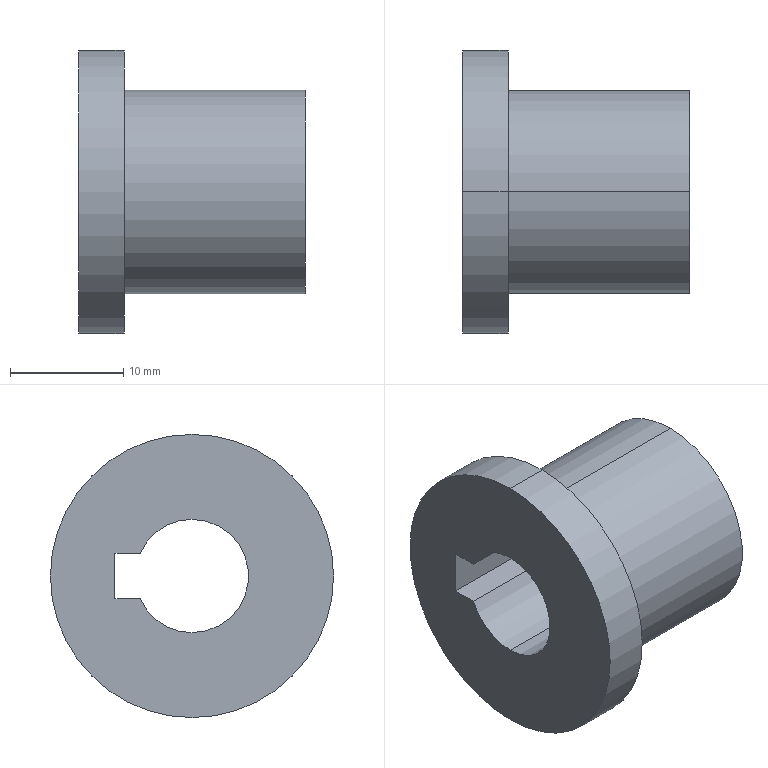Part | SolidWorks | features ICE 1, Revolution 1 | 1 solid | 13 faces | box 20 x 25 x 25 mm | volume 4309 mm3 | cylinder 7 | plane 6 | commonest cylinder face diameters 10 x3 18 x2 25 x2
STEP:
#1=CARTESIAN_POINT('',(4.,0.,12.5));
#2=VERTEX_POINT('',#1);
#3=CARTESIAN_POINT('',(4.,0.,-12.5));
#4=VERTEX_POINT('',#3);
#5=CARTESIAN_POINT('',(4.,0.,0.));
#6=DIRECTION('',(-1.,0.,0.));
#7=DIRECTION('',(0.,0.,1.));
#8=AXIS2_PLACEMENT_3D('',#5,#6,#7);
#9=CIRCLE('',#8,12.5);
#10=EDGE_CURVE('',#2,#4,#9,.T.);
#11=ORIENTED_EDGE('',*,*,#10,.T.);
#12=CARTESIAN_POINT('',(0.,0.,-12.5));
#13=VERTEX_POINT('',#12);
#14=CARTESIAN_POINT('',(0.,0.,-12.5));
#15=DIRECTION('',(-1.,0.,0.));
#16=VECTOR('',#15,1000.);
#17=LINE('',#14,#16);
#18=EDGE_CURVE('',#4,#13,#17,.T.);
#19=ORIENTED_EDGE('',*,*,#18,.T.);
#20=CARTESIAN_POINT('',(0.,0.,12.5));
#21=VERTEX_POINT('',#20);
#22=CARTESIAN_POINT('',(0.,0.,0.));
#23=DIRECTION('',(-1.,0.,0.));
#24=DIRECTION('',(0.,0.,1.));
#25=AXIS2_PLACEMENT_3D('',#22,#23,#24);
#26=CIRCLE('',#25,12.5);
#27=EDGE_CURVE('',#21,#13,#26,.T.);
#28=ORIENTED_EDGE('',*,*,#27,.F.);
#29=CARTESIAN_POINT('',(0.,0.,12.5));
#30=DIRECTION('',(-1.,0.,0.));
#31=VECTOR('',#30,1000.);
#32=LINE('',#29,#31);
#33=EDGE_CURVE('',#2,#21,#32,.T.);
#34=ORIENTED_EDGE('',*,*,#33,.F.);
#35=EDGE_LOOP('',(#11,#19,#28,#34));
#36=FACE_OUTER_BOUND('',#35,.T.);
#37=CARTESIAN_POINT('',(0.,0.,0.));
#38=DIRECTION('',(-1.,0.,0.));
#39=DIRECTION('',(0.,0.,1.));
#40=AXIS2_PLACEMENT_3D('',#37,#38,#39);
#41=CYLINDRICAL_SURFACE('',#40,12.5);
#42=ADVANCED_FACE('',(#36),#41,.T.);
#43=CARTESIAN_POINT('',(20.,0.,9.));
#44=VERTEX_POINT('',#43);
#45=CARTESIAN_POINT('',(20.,0.,-9.));
#46=VERTEX_POINT('',#45);
#47=CARTESIAN_POINT('',(20.,0.,0.));
#48=DIRECTION('',(-1.,0.,0.));
#49=DIRECTION('',(0.,0.,1.));
#50=AXIS2_PLACEMENT_3D('',#47,#48,#49);
#51=CIRCLE('',#50,9.);
#52=EDGE_CURVE('',#44,#46,#51,.T.);
#53=ORIENTED_EDGE('',*,*,#52,.T.);
#54=CARTESIAN_POINT('',(4.,0.,-9.));
#55=VERTEX_POINT('',#54);
#56=CARTESIAN_POINT('',(0.,0.,-9.));
#57=DIRECTION('',(-1.,0.,0.));
#58=VECTOR('',#57,1000.);
#59=LINE('',#56,#58);
#60=EDGE_CURVE('',#46,#55,#59,.T.);
#61=ORIENTED_EDGE('',*,*,#60,.T.);
#62=CARTESIAN_POINT('',(4.,0.,9.));
#63=VERTEX_POINT('',#62);
#64=CARTESIAN_POINT('',(4.,0.,0.));
#65=DIRECTION('',(-1.,0.,0.));
#66=DIRECTION('',(0.,0.,1.));
#67=AXIS2_PLACEMENT_3D('',#64,#65,#66);
#68=CIRCLE('',#67,9.);
#69=EDGE_CURVE('',#63,#55,#68,.T.);
#70=ORIENTED_EDGE('',*,*,#69,.F.);
#71=CARTESIAN_POINT('',(0.,0.,9.));
#72=DIRECTION('',(-1.,0.,0.));
#73=VECTOR('',#72,1000.);
#74=LINE('',#71,#73);
#75=EDGE_CURVE('',#44,#63,#74,.T.);
#76=ORIENTED_EDGE('',*,*,#75,.F.);
#77=EDGE_LOOP('',(#53,#61,#70,#76));
#78=FACE_OUTER_BOUND('',#77,.T.);
#79=CARTESIAN_POINT('',(0.,0.,0.));
#80=DIRECTION('',(-1.,0.,0.));
#81=DIRECTION('',(0.,0.,1.));
#82=AXIS2_PLACEMENT_3D('',#79,#80,#81);
#83=CYLINDRICAL_SURFACE('',#82,9.);
#84=ADVANCED_FACE('',(#78),#83,.T.);
#85=CARTESIAN_POINT('',(20.,0.,-5.));
#86=VERTEX_POINT('',#85);
#87=CARTESIAN_POINT('',(20.,0.,5.));
#88=VERTEX_POINT('',#87);
#89=CARTESIAN_POINT('',(20.,0.,0.));
#90=DIRECTION('',(-1.,0.,0.));
#91=DIRECTION('',(0.,0.,1.));
#92=AXIS2_PLACEMENT_3D('',#89,#90,#91);
#93=CIRCLE('',#92,5.);
#94=EDGE_CURVE('',#86,#88,#93,.T.);
#95=ORIENTED_EDGE('',*,*,#94,.F.);
#96=CARTESIAN_POINT('',(0.,0.,-5.));
#97=VERTEX_POINT('',#96);
#98=CARTESIAN_POINT('',(0.,0.,-5.));
#99=DIRECTION('',(-1.,0.,0.));
#100=VECTOR('',#99,1000.);
#101=LINE('',#98,#100);
#102=EDGE_CURVE('',#86,#97,#101,.T.);
#103=ORIENTED_EDGE('',*,*,#102,.T.);
#104=CARTESIAN_POINT('',(0.,0.,5.));
#105=VERTEX_POINT('',#104);
#106=CARTESIAN_POINT('',(0.,0.,0.));
#107=DIRECTION('',(-1.,0.,0.));
#108=DIRECTION('',(0.,0.,1.));
#109=AXIS2_PLACEMENT_3D('',#106,#107,#108);
#110=CIRCLE('',#109,5.);
#111=EDGE_CURVE('',#97,#105,#110,.T.);
#112=ORIENTED_EDGE('',*,*,#111,.T.);
#113=CARTESIAN_POINT('',(0.,0.,5.));
#114=DIRECTION('',(-1.,0.,0.));
#115=VECTOR('',#114,1000.);
#116=LINE('',#113,#115);
#117=EDGE_CURVE('',#88,#105,#116,.T.);
#118=ORIENTED_EDGE('',*,*,#117,.F.);
#119=EDGE_LOOP('',(#95,#103,#112,#118));
#120=FACE_OUTER_BOUND('',#119,.T.);
#121=CARTESIAN_POINT('',(0.,0.,0.));
#122=DIRECTION('',(-1.,0.,0.));
#123=DIRECTION('',(0.,0.,1.));
#124=AXIS2_PLACEMENT_3D('',#121,#122,#123);
#125=CYLINDRICAL_SURFACE('',#124,5.);
#126=ADVANCED_FACE('',(#120),#125,.F.);
#127=CARTESIAN_POINT('',(20.,4.583,2.));
#128=VERTEX_POINT('',#127);
#129=CARTESIAN_POINT('',(20.,0.,0.));
#130=DIRECTION('',(-1.,0.,0.));
#131=DIRECTION('',(0.,0.,1.));
#132=AXIS2_PLACEMENT_3D('',#129,#130,#131);
#133=CIRCLE('',#132,5.);
#134=EDGE_CURVE('',#88,#128,#133,.T.);
#135=ORIENTED_EDGE('',*,*,#134,.F.);
#136=ORIENTED_EDGE('',*,*,#117,.T.);
#137=CARTESIAN_POINT('',(0.,4.583,2.));
#138=VERTEX_POINT('',#137);
#139=CARTESIAN_POINT('',(0.,0.,0.));
#140=DIRECTION('',(-1.,0.,0.));
#141=DIRECTION('',(0.,0.,1.));
#142=AXIS2_PLACEMENT_3D('',#139,#140,#141);
#143=CIRCLE('',#142,5.);
#144=EDGE_CURVE('',#105,#138,#143,.T.);
#145=ORIENTED_EDGE('',*,*,#144,.T.);
#146=CARTESIAN_POINT('',(0.,4.583,2.));
#147=DIRECTION('',(1.,0.,0.));
#148=VECTOR('',#147,1000.);
#149=LINE('',#146,#148);
#150=EDGE_CURVE('',#138,#128,#149,.T.);
#151=ORIENTED_EDGE('',*,*,#150,.T.);
#152=EDGE_LOOP('',(#135,#136,#145,#151));
#153=FACE_OUTER_BOUND('',#152,.T.);
#154=CARTESIAN_POINT('',(0.,0.,0.));
#155=DIRECTION('',(-1.,0.,0.));
#156=DIRECTION('',(0.,0.,1.));
#157=AXIS2_PLACEMENT_3D('',#154,#155,#156);
#158=CYLINDRICAL_SURFACE('',#157,5.);
#159=ADVANCED_FACE('',(#153),#158,.F.);
#160=CARTESIAN_POINT('',(0.,4.583,-2.));
#161=VERTEX_POINT('',#160);
#162=CARTESIAN_POINT('',(0.,0.,0.));
#163=DIRECTION('',(-1.,0.,0.));
#164=DIRECTION('',(0.,0.,1.));
#165=AXIS2_PLACEMENT_3D('',#162,#163,#164);
#166=CIRCLE('',#165,5.);
#167=EDGE_CURVE('',#161,#97,#166,.T.);
#168=ORIENTED_EDGE('',*,*,#167,.F.);
#169=CARTESIAN_POINT('',(0.,6.8,-2.));
#170=VERTEX_POINT('',#169);
#171=CARTESIAN_POINT('',(0.,0.,-2.));
#172=DIRECTION('',(0.,-1.,0.));
#173=VECTOR('',#172,1000.);
#174=LINE('',#171,#173);
#175=EDGE_CURVE('',#170,#161,#174,.T.);
#176=ORIENTED_EDGE('',*,*,#175,.F.);
#177=CARTESIAN_POINT('',(0.,6.8,2.));
#178=VERTEX_POINT('',#177);
#179=CARTESIAN_POINT('',(0.,6.8,-2.));
#180=DIRECTION('',(0.,0.,-1.));
#181=VECTOR('',#180,1000.);
#182=LINE('',#179,#181);
#183=EDGE_CURVE('',#178,#170,#182,.T.);
#184=ORIENTED_EDGE('',*,*,#183,.F.);
#185=CARTESIAN_POINT('',(0.,0.,2.));
#186=DIRECTION('',(0.,1.,0.));
#187=VECTOR('',#186,1000.);
#188=LINE('',#185,#187);
#189=EDGE_CURVE('',#138,#178,#188,.T.);
#190=ORIENTED_EDGE('',*,*,#189,.F.);
#191=ORIENTED_EDGE('',*,*,#144,.F.);
#192=ORIENTED_EDGE('',*,*,#111,.F.);
#193=EDGE_LOOP('',(#168,#176,#184,#190,#191,#192));
#194=FACE_BOUND('',#193,.T.);
#195=ORIENTED_EDGE('',*,*,#27,.T.);
#196=CARTESIAN_POINT('',(0.,0.,0.));
#197=DIRECTION('',(-1.,0.,0.));
#198=DIRECTION('',(0.,0.,1.));
#199=AXIS2_PLACEMENT_3D('',#196,#197,#198);
#200=CIRCLE('',#199,12.5);
#201=EDGE_CURVE('',#13,#21,#200,.T.);
#202=ORIENTED_EDGE('',*,*,#201,.T.);
#203=EDGE_LOOP('',(#195,#202));
#204=FACE_OUTER_BOUND('',#203,.T.);
#205=CARTESIAN_POINT('',(0.,12.5,0.));
#206=DIRECTION('',(1.,0.,0.));
#207=DIRECTION('',(0.,0.,-1.));
#208=AXIS2_PLACEMENT_3D('',#205,#206,#207);
#209=PLANE('',#208);
#210=ADVANCED_FACE('',(#194,#204),#209,.F.);
#211=ORIENTED_EDGE('',*,*,#102,.F.);
#212=CARTESIAN_POINT('',(20.,4.583,-2.));
#213=VERTEX_POINT('',#212);
#214=CARTESIAN_POINT('',(20.,0.,0.));
#215=DIRECTION('',(-1.,0.,0.));
#216=DIRECTION('',(0.,0.,1.));
#217=AXIS2_PLACEMENT_3D('',#214,#215,#216);
#218=CIRCLE('',#217,5.);
#219=EDGE_CURVE('',#213,#86,#218,.T.);
#220=ORIENTED_EDGE('',*,*,#219,.F.);
#221=CARTESIAN_POINT('',(0.,4.583,-2.));
#222=DIRECTION('',(-1.,0.,0.));
#223=VECTOR('',#222,1000.);
#224=LINE('',#221,#223);
#225=EDGE_CURVE('',#213,#161,#224,.T.);
#226=ORIENTED_EDGE('',*,*,#225,.T.);
#227=ORIENTED_EDGE('',*,*,#167,.T.);
#228=EDGE_LOOP('',(#211,#220,#226,#227));
#229=FACE_OUTER_BOUND('',#228,.T.);
#230=CARTESIAN_POINT('',(0.,0.,0.));
#231=DIRECTION('',(-1.,0.,0.));
#232=DIRECTION('',(0.,0.,1.));
#233=AXIS2_PLACEMENT_3D('',#230,#231,#232);
#234=CYLINDRICAL_SURFACE('',#233,5.);
#235=ADVANCED_FACE('',(#229),#234,.F.);
#236=ORIENTED_EDGE('',*,*,#52,.F.);
#237=CARTESIAN_POINT('',(20.,0.,0.));
#238=DIRECTION('',(-1.,0.,0.));
#239=DIRECTION('',(0.,0.,1.));
#240=AXIS2_PLACEMENT_3D('',#237,#238,#239);
#241=CIRCLE('',#240,9.);
#242=EDGE_CURVE('',#46,#44,#241,.T.);
#243=ORIENTED_EDGE('',*,*,#242,.F.);
#244=EDGE_LOOP('',(#236,#243));
#245=FACE_OUTER_BOUND('',#244,.T.);
#246=CARTESIAN_POINT('',(20.,6.8,2.));
#247=VERTEX_POINT('',#246);
#248=CARTESIAN_POINT('',(20.,6.8,-2.));
#249=VERTEX_POINT('',#248);
#250=CARTESIAN_POINT('',(20.,6.8,-2.));
#251=DIRECTION('',(0.,0.,-1.));
#252=VECTOR('',#251,1000.);
#253=LINE('',#250,#252);
#254=EDGE_CURVE('',#247,#249,#253,.T.);
#255=ORIENTED_EDGE('',*,*,#254,.T.);
#256=CARTESIAN_POINT('',(20.,0.,-2.));
#257=DIRECTION('',(0.,-1.,0.));
#258=VECTOR('',#257,1000.);
#259=LINE('',#256,#258);
#260=EDGE_CURVE('',#249,#213,#259,.T.);
#261=ORIENTED_EDGE('',*,*,#260,.T.);
#262=ORIENTED_EDGE('',*,*,#219,.T.);
#263=ORIENTED_EDGE('',*,*,#94,.T.);
#264=ORIENTED_EDGE('',*,*,#134,.T.);
#265=CARTESIAN_POINT('',(20.,5.,2.));
#266=DIRECTION('',(0.,1.,0.));
#267=VECTOR('',#266,1000.);
#268=LINE('',#265,#267);
#269=EDGE_CURVE('',#128,#247,#268,.T.);
#270=ORIENTED_EDGE('',*,*,#269,.T.);
#271=EDGE_LOOP('',(#255,#261,#262,#263,#264,#270));
#272=FACE_BOUND('',#271,.T.);
#273=CARTESIAN_POINT('',(20.,5.,0.));
#274=DIRECTION('',(-1.,0.,0.));
#275=DIRECTION('',(0.,0.,1.));
#276=AXIS2_PLACEMENT_3D('',#273,#274,#275);
#277=PLANE('',#276);
#278=ADVANCED_FACE('',(#245,#272),#277,.F.);
#279=ORIENTED_EDGE('',*,*,#60,.F.);
#280=ORIENTED_EDGE('',*,*,#242,.T.);
#281=ORIENTED_EDGE('',*,*,#75,.T.);
#282=CARTESIAN_POINT('',(4.,0.,0.));
#283=DIRECTION('',(-1.,0.,0.));
#284=DIRECTION('',(0.,0.,1.));
#285=AXIS2_PLACEMENT_3D('',#282,#283,#284);
#286=CIRCLE('',#285,9.);
#287=EDGE_CURVE('',#55,#63,#286,.T.);
#288=ORIENTED_EDGE('',*,*,#287,.F.);
#289=EDGE_LOOP('',(#279,#280,#281,#288));
#290=FACE_OUTER_BOUND('',#289,.T.);
#291=CARTESIAN_POINT('',(0.,0.,0.));
#292=DIRECTION('',(-1.,0.,0.));
#293=DIRECTION('',(0.,0.,1.));
#294=AXIS2_PLACEMENT_3D('',#291,#292,#293);
#295=CYLINDRICAL_SURFACE('',#294,9.);
#296=ADVANCED_FACE('',(#290),#295,.T.);
#297=ORIENTED_EDGE('',*,*,#10,.F.);
#298=CARTESIAN_POINT('',(4.,0.,0.));
#299=DIRECTION('',(-1.,0.,0.));
#300=DIRECTION('',(0.,0.,1.));
#301=AXIS2_PLACEMENT_3D('',#298,#299,#300);
#302=CIRCLE('',#301,12.5);
#303=EDGE_CURVE('',#4,#2,#302,.T.);
#304=ORIENTED_EDGE('',*,*,#303,.F.);
#305=EDGE_LOOP('',(#297,#304));
#306=FACE_OUTER_BOUND('',#305,.T.);
#307=ORIENTED_EDGE('',*,*,#69,.T.);
#308=ORIENTED_EDGE('',*,*,#287,.T.);
#309=EDGE_LOOP('',(#307,#308));
#310=FACE_BOUND('',#309,.T.);
#311=CARTESIAN_POINT('',(4.,9.,0.));
#312=DIRECTION('',(-1.,0.,0.));
#313=DIRECTION('',(0.,0.,1.));
#314=AXIS2_PLACEMENT_3D('',#311,#312,#313);
#315=PLANE('',#314);
#316=ADVANCED_FACE('',(#306,#310),#315,.F.);
#317=ORIENTED_EDGE('',*,*,#18,.F.);
#318=ORIENTED_EDGE('',*,*,#303,.T.);
#319=ORIENTED_EDGE('',*,*,#33,.T.);
#320=ORIENTED_EDGE('',*,*,#201,.F.);
#321=EDGE_LOOP('',(#317,#318,#319,#320));
#322=FACE_OUTER_BOUND('',#321,.T.);
#323=CARTESIAN_POINT('',(0.,0.,0.));
#324=DIRECTION('',(-1.,0.,0.));
#325=DIRECTION('',(0.,0.,1.));
#326=AXIS2_PLACEMENT_3D('',#323,#324,#325);
#327=CYLINDRICAL_SURFACE('',#326,12.5);
#328=ADVANCED_FACE('',(#322),#327,.T.);
#329=ORIENTED_EDGE('',*,*,#260,.F.);
#330=CARTESIAN_POINT('',(20.,6.8,-2.));
#331=DIRECTION('',(-1.,0.,0.));
#332=VECTOR('',#331,1000.);
#333=LINE('',#330,#332);
#334=EDGE_CURVE('',#249,#170,#333,.T.);
#335=ORIENTED_EDGE('',*,*,#334,.T.);
#336=ORIENTED_EDGE('',*,*,#175,.T.);
#337=ORIENTED_EDGE('',*,*,#225,.F.);
#338=EDGE_LOOP('',(#329,#335,#336,#337));
#339=FACE_OUTER_BOUND('',#338,.T.);
#340=CARTESIAN_POINT('',(20.,0.,-2.));
#341=DIRECTION('',(0.,0.,-1.));
#342=DIRECTION('',(-1.,0.,0.));
#343=AXIS2_PLACEMENT_3D('',#340,#341,#342);
#344=PLANE('',#343);
#345=ADVANCED_FACE('',(#339),#344,.F.);
#346=ORIENTED_EDGE('',*,*,#189,.T.);
#347=CARTESIAN_POINT('',(20.,6.8,2.));
#348=DIRECTION('',(-1.,0.,0.));
#349=VECTOR('',#348,1000.);
#350=LINE('',#347,#349);
#351=EDGE_CURVE('',#247,#178,#350,.T.);
#352=ORIENTED_EDGE('',*,*,#351,.F.);
#353=ORIENTED_EDGE('',*,*,#269,.F.);
#354=ORIENTED_EDGE('',*,*,#150,.F.);
#355=EDGE_LOOP('',(#346,#352,#353,#354));
#356=FACE_OUTER_BOUND('',#355,.T.);
#357=CARTESIAN_POINT('',(20.,0.,2.));
#358=DIRECTION('',(0.,0.,1.));
#359=DIRECTION('',(1.,0.,0.));
#360=AXIS2_PLACEMENT_3D('',#357,#358,#359);
#361=PLANE('',#360);
#362=ADVANCED_FACE('',(#356),#361,.F.);
#363=ORIENTED_EDGE('',*,*,#183,.T.);
#364=ORIENTED_EDGE('',*,*,#334,.F.);
#365=ORIENTED_EDGE('',*,*,#254,.F.);
#366=ORIENTED_EDGE('',*,*,#351,.T.);
#367=EDGE_LOOP('',(#363,#364,#365,#366));
#368=FACE_OUTER_BOUND('',#367,.T.);
#369=CARTESIAN_POINT('',(20.,6.8,-2.));
#370=DIRECTION('',(0.,1.,0.));
#371=DIRECTION('',(0.,0.,1.));
#372=AXIS2_PLACEMENT_3D('',#369,#370,#371);
#373=PLANE('',#372);
#374=ADVANCED_FACE('',(#368),#373,.F.);
#375=CLOSED_SHELL('',(#42,#84,#126,#159,#210,#235,#278,#296,#316,#328,#345,#362,#374));
#376=MANIFOLD_SOLID_BREP('',#375);
#377=CARTESIAN_POINT('',(0.,0.,0.));
#378=DIRECTION('',(0.,0.,1.));
#379=DIRECTION('',(1.,0.,0.));
#380=AXIS2_PLACEMENT_3D('',#377,#378,#379);
#381=(LENGTH_UNIT()NAMED_UNIT(*)SI_UNIT(.MILLI.,.METRE.));
#382=UNCERTAINTY_MEASURE_WITH_UNIT(LENGTH_MEASURE(0.00001),#381,'','');
#383=(NAMED_UNIT(*)PLANE_ANGLE_UNIT()SI_UNIT($,.RADIAN.));
#384=(NAMED_UNIT(*)SI_UNIT($,.STERADIAN.)SOLID_ANGLE_UNIT());
#385=(GEOMETRIC_REPRESENTATION_CONTEXT(3)GLOBAL_UNCERTAINTY_ASSIGNED_CONTEXT((#382))GLOBAL_UNIT_ASSIGNED_CONTEXT((#381,#383,#384))REPRESENTATION_CONTEXT('',''));
#386=ADVANCED_BREP_SHAPE_REPRESENTATION('',(#376,#380),#385);